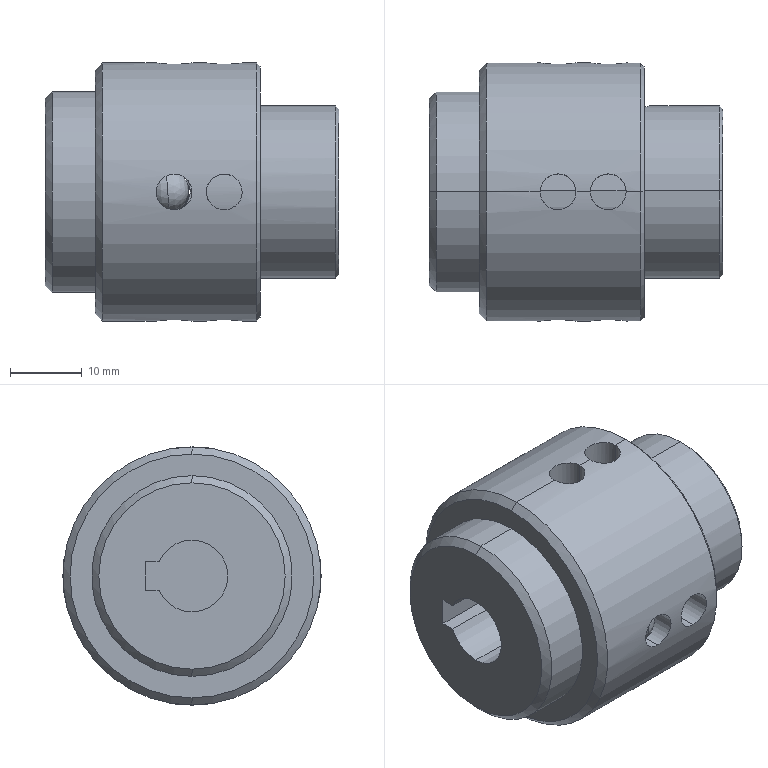Part | SolidWorks | features CompositeCurve 4 | 6 solids | 92 faces | box 41 x 36 x 36 mm | volume 28883 mm3 | cylinder 37 | plane 27 | cone 20 | spline 4 | sphere 4 | commonest cylinder face diameters 5 x18 10 x6 24 x4 4 x3 6.5 x2 28 x2